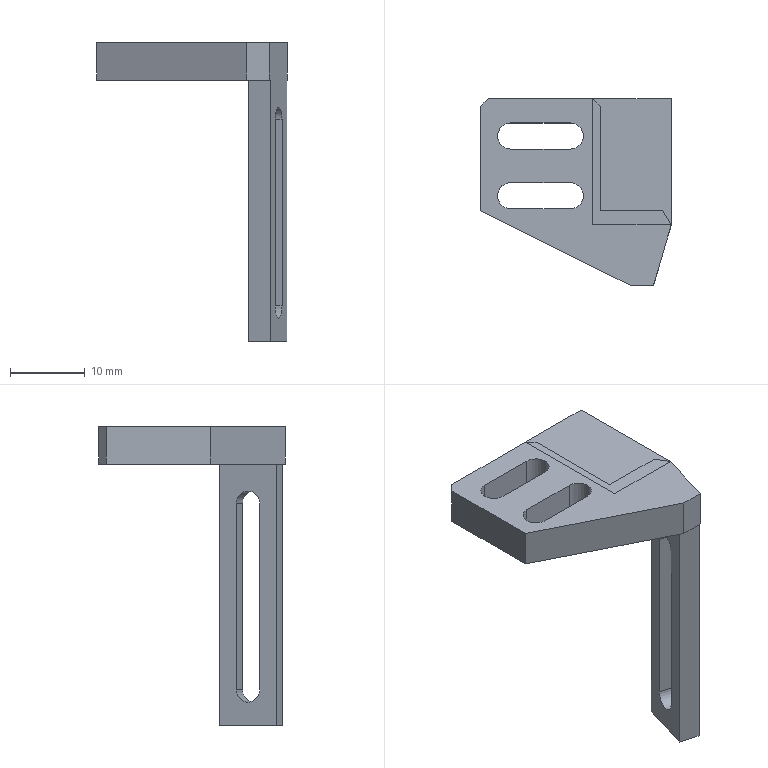Part | NX | 2 solids | 34 faces | box 25.523 x 25 x 40 mm | volume 2991 mm3 | plane 28 | cylinder 6 | commonest cylinder face diameters 3.5 x4 3.3 x2
STEP:
#1=CARTESIAN_POINT('',(12.761,-4.418,0.));
#2=VERTEX_POINT('',#1);
#3=CARTESIAN_POINT('',(2.239,-4.418,0.));
#4=VERTEX_POINT('',#3);
#5=CARTESIAN_POINT('',(7.5,-4.418,0.));
#6=DIRECTION('',(-1.,0.,0.));
#7=VECTOR('',#6,1000.);
#8=LINE('',#5,#7);
#9=EDGE_CURVE('',#2,#4,#8,.T.);
#10=ORIENTED_EDGE('',*,*,#9,.F.);
#11=CARTESIAN_POINT('',(12.761,12.5,0.));
#12=VERTEX_POINT('',#11);
#13=CARTESIAN_POINT('',(12.761,4.041,0.));
#14=DIRECTION('',(0.,-1.,0.));
#15=VECTOR('',#14,1000.);
#16=LINE('',#13,#15);
#17=EDGE_CURVE('',#12,#2,#16,.T.);
#18=ORIENTED_EDGE('',*,*,#17,.F.);
#19=CARTESIAN_POINT('',(2.239,12.5,0.));
#20=VERTEX_POINT('',#19);
#21=CARTESIAN_POINT('',(7.5,12.5,0.));
#22=DIRECTION('',(1.,0.,0.));
#23=VECTOR('',#22,1000.);
#24=LINE('',#21,#23);
#25=EDGE_CURVE('',#20,#12,#24,.T.);
#26=ORIENTED_EDGE('',*,*,#25,.F.);
#27=CARTESIAN_POINT('',(2.239,4.041,0.));
#28=DIRECTION('',(0.,1.,0.));
#29=VECTOR('',#28,1000.);
#30=LINE('',#27,#29);
#31=EDGE_CURVE('',#4,#20,#30,.T.);
#32=ORIENTED_EDGE('',*,*,#31,.F.);
#33=EDGE_LOOP('',(#10,#18,#26,#32));
#34=FACE_BOUND('',#33,.T.);
#35=CARTESIAN_POINT('',(7.5,4.041,0.));
#36=DIRECTION('',(0.,0.,1.));
#37=DIRECTION('',(1.,0.,0.));
#38=AXIS2_PLACEMENT_3D('',#35,#36,#37);
#39=PLANE('',#38);
#40=ADVANCED_FACE('',(#34),#39,.T.);
#41=CARTESIAN_POINT('',(12.761,-4.418,-5.));
#42=VERTEX_POINT('',#41);
#43=CARTESIAN_POINT('',(12.761,-4.418,-5.));
#44=DIRECTION('',(0.,0.,1.));
#45=VECTOR('',#44,1000.);
#46=LINE('',#43,#45);
#47=EDGE_CURVE('',#42,#2,#46,.T.);
#48=ORIENTED_EDGE('',*,*,#47,.T.);
#49=ORIENTED_EDGE('',*,*,#9,.T.);
#50=CARTESIAN_POINT('',(2.239,-4.418,-5.));
#51=VERTEX_POINT('',#50);
#52=CARTESIAN_POINT('',(2.239,-4.418,-5.));
#53=DIRECTION('',(0.,0.,1.));
#54=VECTOR('',#53,1000.);
#55=LINE('',#52,#54);
#56=EDGE_CURVE('',#51,#4,#55,.T.);
#57=ORIENTED_EDGE('',*,*,#56,.F.);
#58=CARTESIAN_POINT('',(7.5,-4.418,-5.));
#59=DIRECTION('',(1.,0.,0.));
#60=VECTOR('',#59,1000.);
#61=LINE('',#58,#60);
#62=EDGE_CURVE('',#51,#42,#61,.T.);
#63=ORIENTED_EDGE('',*,*,#62,.T.);
#64=EDGE_LOOP('',(#48,#49,#57,#63));
#65=FACE_BOUND('',#64,.T.);
#66=CARTESIAN_POINT('',(7.5,-4.418,-5.));
#67=DIRECTION('',(0.,-1.,0.));
#68=DIRECTION('',(0.,0.,-1.));
#69=AXIS2_PLACEMENT_3D('',#66,#67,#68);
#70=PLANE('',#69);
#71=ADVANCED_FACE('',(#65),#70,.T.);
#72=ORIENTED_EDGE('',*,*,#56,.T.);
#73=ORIENTED_EDGE('',*,*,#31,.T.);
#74=CARTESIAN_POINT('',(2.239,12.5,-5.));
#75=VERTEX_POINT('',#74);
#76=CARTESIAN_POINT('',(2.239,12.5,-5.));
#77=DIRECTION('',(0.,0.,1.));
#78=VECTOR('',#77,1000.);
#79=LINE('',#76,#78);
#80=EDGE_CURVE('',#75,#20,#79,.T.);
#81=ORIENTED_EDGE('',*,*,#80,.F.);
#82=CARTESIAN_POINT('',(2.239,4.041,-5.));
#83=DIRECTION('',(0.,-1.,0.));
#84=VECTOR('',#83,1000.);
#85=LINE('',#82,#84);
#86=EDGE_CURVE('',#75,#51,#85,.T.);
#87=ORIENTED_EDGE('',*,*,#86,.T.);
#88=EDGE_LOOP('',(#72,#73,#81,#87));
#89=FACE_BOUND('',#88,.T.);
#90=CARTESIAN_POINT('',(2.239,4.041,-5.));
#91=DIRECTION('',(-1.,0.,0.));
#92=DIRECTION('',(0.,0.,1.));
#93=AXIS2_PLACEMENT_3D('',#90,#91,#92);
#94=PLANE('',#93);
#95=ADVANCED_FACE('',(#89),#94,.T.);
#96=ORIENTED_EDGE('',*,*,#80,.T.);
#97=ORIENTED_EDGE('',*,*,#25,.T.);
#98=CARTESIAN_POINT('',(12.761,12.5,-5.));
#99=VERTEX_POINT('',#98);
#100=CARTESIAN_POINT('',(12.761,12.5,-5.));
#101=DIRECTION('',(0.,0.,1.));
#102=VECTOR('',#101,1000.);
#103=LINE('',#100,#102);
#104=EDGE_CURVE('',#99,#12,#103,.T.);
#105=ORIENTED_EDGE('',*,*,#104,.F.);
#106=CARTESIAN_POINT('',(7.5,12.5,-5.));
#107=DIRECTION('',(-1.,0.,0.));
#108=VECTOR('',#107,1000.);
#109=LINE('',#106,#108);
#110=EDGE_CURVE('',#99,#75,#109,.T.);
#111=ORIENTED_EDGE('',*,*,#110,.T.);
#112=EDGE_LOOP('',(#96,#97,#105,#111));
#113=FACE_BOUND('',#112,.T.);
#114=CARTESIAN_POINT('',(7.5,12.5,-5.));
#115=DIRECTION('',(0.,1.,0.));
#116=DIRECTION('',(0.,0.,1.));
#117=AXIS2_PLACEMENT_3D('',#114,#115,#116);
#118=PLANE('',#117);
#119=ADVANCED_FACE('',(#113),#118,.T.);
#120=CARTESIAN_POINT('',(12.761,4.041,-5.));
#121=DIRECTION('',(0.,1.,0.));
#122=VECTOR('',#121,1000.);
#123=LINE('',#120,#122);
#124=EDGE_CURVE('',#42,#99,#123,.T.);
#125=ORIENTED_EDGE('',*,*,#124,.F.);
#126=ORIENTED_EDGE('',*,*,#62,.F.);
#127=ORIENTED_EDGE('',*,*,#86,.F.);
#128=ORIENTED_EDGE('',*,*,#110,.F.);
#129=EDGE_LOOP('',(#125,#126,#127,#128));
#130=FACE_BOUND('',#129,.T.);
#131=CARTESIAN_POINT('',(7.5,4.041,-5.));
#132=DIRECTION('',(0.,0.,-1.));
#133=DIRECTION('',(-1.,0.,0.));
#134=AXIS2_PLACEMENT_3D('',#131,#132,#133);
#135=PLANE('',#134);
#136=ADVANCED_FACE('',(#130),#135,.T.);
#137=ORIENTED_EDGE('',*,*,#124,.T.);
#138=ORIENTED_EDGE('',*,*,#104,.T.);
#139=ORIENTED_EDGE('',*,*,#17,.T.);
#140=ORIENTED_EDGE('',*,*,#47,.F.);
#141=EDGE_LOOP('',(#137,#138,#139,#140));
#142=FACE_BOUND('',#141,.T.);
#143=CARTESIAN_POINT('',(12.761,4.041,-5.));
#144=DIRECTION('',(1.,0.,0.));
#145=DIRECTION('',(0.,0.,-1.));
#146=AXIS2_PLACEMENT_3D('',#143,#144,#145);
#147=PLANE('',#146);
#148=ADVANCED_FACE('',(#142),#147,.T.);
#149=CLOSED_SHELL('',(#40,#71,#95,#119,#136,#148));
#150=MANIFOLD_SOLID_BREP('',#149);
#151=CARTESIAN_POINT('',(10.367,-12.5,0.));
#152=VERTEX_POINT('',#151);
#153=CARTESIAN_POINT('',(7.239,-12.5,0.));
#154=VERTEX_POINT('',#153);
#155=CARTESIAN_POINT('',(-12.761,-12.5,0.));
#156=DIRECTION('',(-1.,0.,0.));
#157=VECTOR('',#156,1000.);
#158=LINE('',#155,#157);
#159=EDGE_CURVE('',#152,#154,#158,.T.);
#160=ORIENTED_EDGE('',*,*,#159,.T.);
#161=CARTESIAN_POINT('',(7.239,-12.5,-5.));
#162=VERTEX_POINT('',#161);
#163=CARTESIAN_POINT('',(7.239,-12.5,-5.));
#164=DIRECTION('',(0.,0.,-1.));
#165=VECTOR('',#164,1000.);
#166=LINE('',#163,#165);
#167=EDGE_CURVE('',#154,#162,#166,.T.);
#168=ORIENTED_EDGE('',*,*,#167,.T.);
#169=CARTESIAN_POINT('',(10.367,-12.5,-5.));
#170=VERTEX_POINT('',#169);
#171=CARTESIAN_POINT('',(-12.761,-12.5,-5.));
#172=DIRECTION('',(-1.,0.,0.));
#173=VECTOR('',#172,1000.);
#174=LINE('',#171,#173);
#175=EDGE_CURVE('',#170,#162,#174,.T.);
#176=ORIENTED_EDGE('',*,*,#175,.F.);
#177=CARTESIAN_POINT('',(10.367,-12.5,0.));
#178=DIRECTION('',(0.,0.,-1.));
#179=VECTOR('',#178,1000.);
#180=LINE('',#177,#179);
#181=EDGE_CURVE('',#152,#170,#180,.T.);
#182=ORIENTED_EDGE('',*,*,#181,.F.);
#183=EDGE_LOOP('',(#160,#168,#176,#182));
#184=FACE_BOUND('',#183,.T.);
#185=CARTESIAN_POINT('',(-12.761,-12.5,-5.));
#186=DIRECTION('',(0.,1.,0.));
#187=DIRECTION('',(-1.,0.,0.));
#188=AXIS2_PLACEMENT_3D('',#185,#186,#187);
#189=PLANE('',#188);
#190=ADVANCED_FACE('',(#184),#189,.F.);
#191=CARTESIAN_POINT('',(8.251,-9.082,-10.25));
#192=VERTEX_POINT('',#191);
#193=CARTESIAN_POINT('',(8.251,-9.082,-35.25));
#194=VERTEX_POINT('',#193);
#195=CARTESIAN_POINT('',(8.251,-9.082,-35.));
#196=DIRECTION('',(0.,0.,-1.));
#197=VECTOR('',#196,1000.);
#198=LINE('',#195,#197);
#199=EDGE_CURVE('',#192,#194,#198,.T.);
#200=ORIENTED_EDGE('',*,*,#199,.T.);
#201=CARTESIAN_POINT('',(9.188,-5.918,-35.25));
#202=VERTEX_POINT('',#201);
#203=CARTESIAN_POINT('',(8.72,-7.5,-35.25));
#204=DIRECTION('',(0.9588,-0.284,0.));
#205=DIRECTION('',(-0.284,-0.9588,0.));
#206=AXIS2_PLACEMENT_3D('',#203,#204,#205);
#207=CIRCLE('',#206,1.65);
#208=EDGE_CURVE('',#194,#202,#207,.T.);
#209=ORIENTED_EDGE('',*,*,#208,.T.);
#210=CARTESIAN_POINT('',(9.188,-5.918,-10.25));
#211=VERTEX_POINT('',#210);
#212=CARTESIAN_POINT('',(9.188,-5.918,-35.));
#213=DIRECTION('',(0.,0.,1.));
#214=VECTOR('',#213,1000.);
#215=LINE('',#212,#214);
#216=EDGE_CURVE('',#202,#211,#215,.T.);
#217=ORIENTED_EDGE('',*,*,#216,.T.);
#218=CARTESIAN_POINT('',(8.72,-7.5,-10.25));
#219=DIRECTION('',(0.9588,-0.284,0.));
#220=DIRECTION('',(-0.284,-0.9588,0.));
#221=AXIS2_PLACEMENT_3D('',#218,#219,#220);
#222=CIRCLE('',#221,1.65);
#223=EDGE_CURVE('',#211,#192,#222,.T.);
#224=ORIENTED_EDGE('',*,*,#223,.T.);
#225=EDGE_LOOP('',(#200,#209,#217,#224));
#226=FACE_BOUND('',#225,.T.);
#227=CARTESIAN_POINT('',(7.593,-11.302,-5.));
#228=VERTEX_POINT('',#227);
#229=CARTESIAN_POINT('',(9.846,-3.698,-5.));
#230=VERTEX_POINT('',#229);
#231=CARTESIAN_POINT('',(13.163,7.5,-5.));
#232=DIRECTION('',(0.284,0.9588,0.));
#233=VECTOR('',#232,1000.);
#234=LINE('',#231,#233);
#235=EDGE_CURVE('',#228,#230,#234,.T.);
#236=ORIENTED_EDGE('',*,*,#235,.T.);
#237=CARTESIAN_POINT('',(9.846,-3.698,-40.));
#238=VERTEX_POINT('',#237);
#239=CARTESIAN_POINT('',(9.846,-3.698,0.));
#240=DIRECTION('',(0.,0.,1.));
#241=VECTOR('',#240,1000.);
#242=LINE('',#239,#241);
#243=EDGE_CURVE('',#238,#230,#242,.T.);
#244=ORIENTED_EDGE('',*,*,#243,.F.);
#245=CARTESIAN_POINT('',(7.593,-11.302,-40.));
#246=VERTEX_POINT('',#245);
#247=CARTESIAN_POINT('',(9.856,-3.665,-40.));
#248=DIRECTION('',(-0.284,-0.9588,0.));
#249=VECTOR('',#248,1000.);
#250=LINE('',#247,#249);
#251=EDGE_CURVE('',#238,#246,#250,.T.);
#252=ORIENTED_EDGE('',*,*,#251,.T.);
#253=CARTESIAN_POINT('',(7.593,-11.302,0.));
#254=DIRECTION('',(0.,0.,1.));
#255=VECTOR('',#254,1000.);
#256=LINE('',#253,#255);
#257=EDGE_CURVE('',#246,#228,#256,.T.);
#258=ORIENTED_EDGE('',*,*,#257,.T.);
#259=EDGE_LOOP('',(#236,#244,#252,#258));
#260=FACE_BOUND('',#259,.T.);
#261=CARTESIAN_POINT('',(13.163,7.5,-35.));
#262=DIRECTION('',(0.9588,-0.284,0.));
#263=DIRECTION('',(0.284,0.9588,0.));
#264=AXIS2_PLACEMENT_3D('',#261,#262,#263);
#265=PLANE('',#264);
#266=ADVANCED_FACE('',(#226,#260),#265,.F.);
#267=CARTESIAN_POINT('',(12.065,-6.77,-35.25));
#268=VERTEX_POINT('',#267);
#269=CARTESIAN_POINT('',(12.065,-6.77,-10.25));
#270=VERTEX_POINT('',#269);
#271=CARTESIAN_POINT('',(12.065,-6.77,-35.25));
#272=DIRECTION('',(0.,0.,1.));
#273=VECTOR('',#272,1000.);
#274=LINE('',#271,#273);
#275=EDGE_CURVE('',#268,#270,#274,.T.);
#276=ORIENTED_EDGE('',*,*,#275,.F.);
#277=CARTESIAN_POINT('',(11.127,-9.934,-35.25));
#278=VERTEX_POINT('',#277);
#279=CARTESIAN_POINT('',(11.596,-8.352,-35.25));
#280=DIRECTION('',(0.9588,-0.284,0.));
#281=DIRECTION('',(-0.284,-0.9588,0.));
#282=AXIS2_PLACEMENT_3D('',#279,#280,#281);
#283=CIRCLE('',#282,1.65);
#284=EDGE_CURVE('',#278,#268,#283,.T.);
#285=ORIENTED_EDGE('',*,*,#284,.F.);
#286=CARTESIAN_POINT('',(11.127,-9.934,-10.25));
#287=VERTEX_POINT('',#286);
#288=CARTESIAN_POINT('',(11.127,-9.934,-35.25));
#289=DIRECTION('',(0.,0.,-1.));
#290=VECTOR('',#289,1000.);
#291=LINE('',#288,#290);
#292=EDGE_CURVE('',#287,#278,#291,.T.);
#293=ORIENTED_EDGE('',*,*,#292,.F.);
#294=CARTESIAN_POINT('',(11.596,-8.352,-10.25));
#295=DIRECTION('',(0.9588,-0.284,0.));
#296=DIRECTION('',(-0.284,-0.9588,0.));
#297=AXIS2_PLACEMENT_3D('',#294,#295,#296);
#298=CIRCLE('',#297,1.65);
#299=EDGE_CURVE('',#270,#287,#298,.T.);
#300=ORIENTED_EDGE('',*,*,#299,.F.);
#301=EDGE_LOOP('',(#276,#285,#293,#300));
#302=FACE_BOUND('',#301,.T.);
#303=CARTESIAN_POINT('',(12.761,-4.418,-5.));
#304=VERTEX_POINT('',#303);
#305=CARTESIAN_POINT('',(12.722,-4.55,-5.));
#306=VERTEX_POINT('',#305);
#307=CARTESIAN_POINT('',(13.33,-2.5,-5.));
#308=DIRECTION('',(0.284,0.9588,0.));
#309=VECTOR('',#308,1000.);
#310=LINE('',#307,#309);
#311=EDGE_CURVE('',#304,#306,#310,.F.);
#312=ORIENTED_EDGE('',*,*,#311,.F.);
#313=CARTESIAN_POINT('',(12.761,-4.418,0.));
#314=VERTEX_POINT('',#313);
#315=CARTESIAN_POINT('',(12.761,-4.418,0.));
#316=DIRECTION('',(0.,0.,1.));
#317=VECTOR('',#316,1000.);
#318=LINE('',#315,#317);
#319=EDGE_CURVE('',#304,#314,#318,.T.);
#320=ORIENTED_EDGE('',*,*,#319,.T.);
#321=CARTESIAN_POINT('',(13.33,-2.5,0.));
#322=DIRECTION('',(0.284,0.9588,0.));
#323=VECTOR('',#322,1000.);
#324=LINE('',#321,#323);
#325=EDGE_CURVE('',#152,#314,#324,.T.);
#326=ORIENTED_EDGE('',*,*,#325,.F.);
#327=ORIENTED_EDGE('',*,*,#181,.T.);
#328=CARTESIAN_POINT('',(10.47,-12.154,-5.));
#329=VERTEX_POINT('',#328);
#330=CARTESIAN_POINT('',(13.33,-2.5,-5.));
#331=DIRECTION('',(-0.284,-0.9588,0.));
#332=VECTOR('',#331,1000.);
#333=LINE('',#330,#332);
#334=EDGE_CURVE('',#170,#329,#333,.F.);
#335=ORIENTED_EDGE('',*,*,#334,.T.);
#336=CARTESIAN_POINT('',(10.47,-12.154,-40.));
#337=VERTEX_POINT('',#336);
#338=CARTESIAN_POINT('',(10.47,-12.154,0.));
#339=DIRECTION('',(0.,0.,1.));
#340=VECTOR('',#339,1000.);
#341=LINE('',#338,#340);
#342=EDGE_CURVE('',#337,#329,#341,.T.);
#343=ORIENTED_EDGE('',*,*,#342,.F.);
#344=CARTESIAN_POINT('',(12.722,-4.55,-40.));
#345=VERTEX_POINT('',#344);
#346=CARTESIAN_POINT('',(12.732,-4.517,-40.));
#347=DIRECTION('',(0.284,0.9588,0.));
#348=VECTOR('',#347,1000.);
#349=LINE('',#346,#348);
#350=EDGE_CURVE('',#337,#345,#349,.T.);
#351=ORIENTED_EDGE('',*,*,#350,.T.);
#352=CARTESIAN_POINT('',(12.722,-4.55,0.));
#353=DIRECTION('',(0.,0.,1.));
#354=VECTOR('',#353,1000.);
#355=LINE('',#352,#354);
#356=EDGE_CURVE('',#345,#306,#355,.T.);
#357=ORIENTED_EDGE('',*,*,#356,.T.);
#358=EDGE_LOOP('',(#312,#320,#326,#327,#335,#343,#351,#357));
#359=FACE_BOUND('',#358,.T.);
#360=CARTESIAN_POINT('',(13.33,-2.5,0.));
#361=DIRECTION('',(-0.9588,0.284,0.));
#362=DIRECTION('',(-0.284,-0.9588,0.));
#363=AXIS2_PLACEMENT_3D('',#360,#361,#362);
#364=PLANE('',#363);
#365=ADVANCED_FACE('',(#302,#359),#364,.F.);
#366=CARTESIAN_POINT('',(-0.7615,-2.25,-5.));
#367=VERTEX_POINT('',#366);
#368=CARTESIAN_POINT('',(-8.761,-2.25,-5.));
#369=VERTEX_POINT('',#368);
#370=CARTESIAN_POINT('',(-0.7615,-2.25,-5.));
#371=DIRECTION('',(-1.,0.,0.));
#372=VECTOR('',#371,1000.);
#373=LINE('',#370,#372);
#374=EDGE_CURVE('',#367,#369,#373,.T.);
#375=ORIENTED_EDGE('',*,*,#374,.F.);
#376=CARTESIAN_POINT('',(-0.7615,1.25,-5.));
#377=VERTEX_POINT('',#376);
#378=CARTESIAN_POINT('',(-0.7615,-0.5,-5.));
#379=DIRECTION('',(0.,0.,-1.));
#380=DIRECTION('',(0.,-1.,0.));
#381=AXIS2_PLACEMENT_3D('',#378,#379,#380);
#382=CIRCLE('',#381,1.75);
#383=EDGE_CURVE('',#377,#367,#382,.T.);
#384=ORIENTED_EDGE('',*,*,#383,.F.);
#385=CARTESIAN_POINT('',(-8.761,1.25,-5.));
#386=VERTEX_POINT('',#385);
#387=CARTESIAN_POINT('',(-0.7615,1.25,-5.));
#388=DIRECTION('',(1.,0.,0.));
#389=VECTOR('',#388,1000.);
#390=LINE('',#387,#389);
#391=EDGE_CURVE('',#386,#377,#390,.T.);
#392=ORIENTED_EDGE('',*,*,#391,.F.);
#393=CARTESIAN_POINT('',(-8.761,-0.5,-5.));
#394=DIRECTION('',(0.,0.,-1.));
#395=DIRECTION('',(0.,-1.,0.));
#396=AXIS2_PLACEMENT_3D('',#393,#394,#395);
#397=CIRCLE('',#396,1.75);
#398=EDGE_CURVE('',#369,#386,#397,.T.);
#399=ORIENTED_EDGE('',*,*,#398,.F.);
#400=EDGE_LOOP('',(#375,#384,#392,#399));
#401=FACE_BOUND('',#400,.T.);
#402=CARTESIAN_POINT('',(-0.7615,5.75,-5.));
#403=VERTEX_POINT('',#402);
#404=CARTESIAN_POINT('',(-8.761,5.75,-5.));
#405=VERTEX_POINT('',#404);
#406=CARTESIAN_POINT('',(-0.7615,5.75,-5.));
#407=DIRECTION('',(-1.,0.,0.));
#408=VECTOR('',#407,1000.);
#409=LINE('',#406,#408);
#410=EDGE_CURVE('',#403,#405,#409,.T.);
#411=ORIENTED_EDGE('',*,*,#410,.F.);
#412=CARTESIAN_POINT('',(-0.7615,9.25,-5.));
#413=VERTEX_POINT('',#412);
#414=CARTESIAN_POINT('',(-0.7615,7.5,-5.));
#415=DIRECTION('',(0.,0.,-1.));
#416=DIRECTION('',(0.,-1.,0.));
#417=AXIS2_PLACEMENT_3D('',#414,#415,#416);
#418=CIRCLE('',#417,1.75);
#419=EDGE_CURVE('',#413,#403,#418,.T.);
#420=ORIENTED_EDGE('',*,*,#419,.F.);
#421=CARTESIAN_POINT('',(-8.761,9.25,-5.));
#422=VERTEX_POINT('',#421);
#423=CARTESIAN_POINT('',(-0.7615,9.25,-5.));
#424=DIRECTION('',(1.,0.,0.));
#425=VECTOR('',#424,1000.);
#426=LINE('',#423,#425);
#427=EDGE_CURVE('',#422,#413,#426,.T.);
#428=ORIENTED_EDGE('',*,*,#427,.F.);
#429=CARTESIAN_POINT('',(-8.761,7.5,-5.));
#430=DIRECTION('',(0.,0.,-1.));
#431=DIRECTION('',(0.,-1.,0.));
#432=AXIS2_PLACEMENT_3D('',#429,#430,#431);
#433=CIRCLE('',#432,1.75);
#434=EDGE_CURVE('',#405,#422,#433,.T.);
#435=ORIENTED_EDGE('',*,*,#434,.F.);
#436=EDGE_LOOP('',(#411,#420,#428,#435));
#437=FACE_BOUND('',#436,.T.);
#438=ORIENTED_EDGE('',*,*,#175,.T.);
#439=CARTESIAN_POINT('',(-12.761,-2.5,-5.));
#440=VERTEX_POINT('',#439);
#441=CARTESIAN_POINT('',(-12.761,-2.5,-5.));
#442=DIRECTION('',(-0.8944,0.4472,0.));
#443=VECTOR('',#442,1000.);
#444=LINE('',#441,#443);
#445=EDGE_CURVE('',#162,#440,#444,.T.);
#446=ORIENTED_EDGE('',*,*,#445,.T.);
#447=CARTESIAN_POINT('',(-12.761,11.5,-5.));
#448=VERTEX_POINT('',#447);
#449=CARTESIAN_POINT('',(-12.761,12.5,-5.));
#450=DIRECTION('',(0.,1.,0.));
#451=VECTOR('',#450,1000.);
#452=LINE('',#449,#451);
#453=EDGE_CURVE('',#440,#448,#452,.T.);
#454=ORIENTED_EDGE('',*,*,#453,.T.);
#455=CARTESIAN_POINT('',(-11.761,12.5,-5.));
#456=VERTEX_POINT('',#455);
#457=CARTESIAN_POINT('',(-11.761,12.5,-5.));
#458=DIRECTION('',(0.7071,0.7071,0.));
#459=VECTOR('',#458,1000.);
#460=LINE('',#457,#459);
#461=EDGE_CURVE('',#448,#456,#460,.T.);
#462=ORIENTED_EDGE('',*,*,#461,.T.);
#463=CARTESIAN_POINT('',(2.239,12.5,-5.));
#464=VERTEX_POINT('',#463);
#465=CARTESIAN_POINT('',(17.239,12.5,-5.));
#466=DIRECTION('',(1.,0.,0.));
#467=VECTOR('',#466,1000.);
#468=LINE('',#465,#467);
#469=EDGE_CURVE('',#456,#464,#468,.T.);
#470=ORIENTED_EDGE('',*,*,#469,.T.);
#471=CARTESIAN_POINT('',(3.239,11.5,-5.));
#472=VERTEX_POINT('',#471);
#473=CARTESIAN_POINT('',(2.239,12.5,-5.));
#474=DIRECTION('',(0.7071,-0.7071,0.));
#475=VECTOR('',#474,1000.);
#476=LINE('',#473,#475);
#477=EDGE_CURVE('',#464,#472,#476,.T.);
#478=ORIENTED_EDGE('',*,*,#477,.T.);
#479=CARTESIAN_POINT('',(3.239,-2.5,-5.));
#480=VERTEX_POINT('',#479);
#481=CARTESIAN_POINT('',(3.239,-12.5,-5.));
#482=DIRECTION('',(0.,-1.,0.));
#483=VECTOR('',#482,1000.);
#484=LINE('',#481,#483);
#485=EDGE_CURVE('',#472,#480,#484,.T.);
#486=ORIENTED_EDGE('',*,*,#485,.T.);
#487=CARTESIAN_POINT('',(11.586,-2.5,-5.));
#488=VERTEX_POINT('',#487);
#489=CARTESIAN_POINT('',(-12.761,-2.5,-5.));
#490=DIRECTION('',(1.,0.,0.));
#491=VECTOR('',#490,1000.);
#492=LINE('',#489,#491);
#493=EDGE_CURVE('',#480,#488,#492,.T.);
#494=ORIENTED_EDGE('',*,*,#493,.T.);
#495=CARTESIAN_POINT('',(11.586,-2.5,-5.));
#496=DIRECTION('',(0.5225,-0.8526,0.));
#497=VECTOR('',#496,1000.);
#498=LINE('',#495,#497);
#499=EDGE_CURVE('',#488,#304,#498,.T.);
#500=ORIENTED_EDGE('',*,*,#499,.T.);
#501=ORIENTED_EDGE('',*,*,#311,.T.);
#502=CARTESIAN_POINT('',(17.516,-5.97,-5.));
#503=DIRECTION('',(-0.9588,0.284,0.));
#504=VECTOR('',#503,1000.);
#505=LINE('',#502,#504);
#506=EDGE_CURVE('',#306,#230,#505,.T.);
#507=ORIENTED_EDGE('',*,*,#506,.T.);
#508=ORIENTED_EDGE('',*,*,#235,.F.);
#509=CARTESIAN_POINT('',(15.264,-13.574,-5.));
#510=DIRECTION('',(-0.9588,0.284,0.));
#511=VECTOR('',#510,1000.);
#512=LINE('',#509,#511);
#513=EDGE_CURVE('',#329,#228,#512,.T.);
#514=ORIENTED_EDGE('',*,*,#513,.F.);
#515=ORIENTED_EDGE('',*,*,#334,.F.);
#516=EDGE_LOOP('',(#438,#446,#454,#462,#470,#478,#486,#494,#500,#501,#507,#508,#514,#515));
#517=FACE_BOUND('',#516,.T.);
#518=CARTESIAN_POINT('',(-12.761,-12.5,-5.));
#519=DIRECTION('',(0.,0.,1.));
#520=DIRECTION('',(0.,-1.,0.));
#521=AXIS2_PLACEMENT_3D('',#518,#519,#520);
#522=PLANE('',#521);
#523=ADVANCED_FACE('',(#401,#437,#517),#522,.F.);
#524=ORIENTED_EDGE('',*,*,#453,.F.);
#525=CARTESIAN_POINT('',(-12.761,-2.5,0.));
#526=VERTEX_POINT('',#525);
#527=CARTESIAN_POINT('',(-12.761,-2.5,-5.));
#528=DIRECTION('',(0.,0.,1.));
#529=VECTOR('',#528,1000.);
#530=LINE('',#527,#529);
#531=EDGE_CURVE('',#440,#526,#530,.T.);
#532=ORIENTED_EDGE('',*,*,#531,.T.);
#533=CARTESIAN_POINT('',(-12.761,11.5,0.));
#534=VERTEX_POINT('',#533);
#535=CARTESIAN_POINT('',(-12.761,12.5,0.));
#536=DIRECTION('',(0.,1.,0.));
#537=VECTOR('',#536,1000.);
#538=LINE('',#535,#537);
#539=EDGE_CURVE('',#526,#534,#538,.T.);
#540=ORIENTED_EDGE('',*,*,#539,.T.);
#541=CARTESIAN_POINT('',(-12.761,11.5,-5.));
#542=DIRECTION('',(0.,0.,-1.));
#543=VECTOR('',#542,1000.);
#544=LINE('',#541,#543);
#545=EDGE_CURVE('',#534,#448,#544,.T.);
#546=ORIENTED_EDGE('',*,*,#545,.T.);
#547=EDGE_LOOP('',(#524,#532,#540,#546));
#548=FACE_BOUND('',#547,.T.);
#549=CARTESIAN_POINT('',(-12.761,12.5,-5.));
#550=DIRECTION('',(1.,0.,0.));
#551=DIRECTION('',(0.,1.,0.));
#552=AXIS2_PLACEMENT_3D('',#549,#550,#551);
#553=PLANE('',#552);
#554=ADVANCED_FACE('',(#548),#553,.F.);
#555=ORIENTED_EDGE('',*,*,#469,.F.);
#556=CARTESIAN_POINT('',(-11.761,12.5,0.));
#557=VERTEX_POINT('',#556);
#558=CARTESIAN_POINT('',(-11.761,12.5,-5.));
#559=DIRECTION('',(0.,0.,1.));
#560=VECTOR('',#559,1000.);
#561=LINE('',#558,#560);
#562=EDGE_CURVE('',#456,#557,#561,.T.);
#563=ORIENTED_EDGE('',*,*,#562,.T.);
#564=CARTESIAN_POINT('',(2.239,12.5,0.));
#565=VERTEX_POINT('',#564);
#566=CARTESIAN_POINT('',(17.239,12.5,0.));
#567=DIRECTION('',(1.,0.,0.));
#568=VECTOR('',#567,1000.);
#569=LINE('',#566,#568);
#570=EDGE_CURVE('',#557,#565,#569,.T.);
#571=ORIENTED_EDGE('',*,*,#570,.T.);
#572=CARTESIAN_POINT('',(2.239,12.5,-5.));
#573=DIRECTION('',(0.,0.,-1.));
#574=VECTOR('',#573,1000.);
#575=LINE('',#572,#574);
#576=EDGE_CURVE('',#565,#464,#575,.T.);
#577=ORIENTED_EDGE('',*,*,#576,.T.);
#578=EDGE_LOOP('',(#555,#563,#571,#577));
#579=FACE_BOUND('',#578,.T.);
#580=CARTESIAN_POINT('',(17.239,12.5,-5.));
#581=DIRECTION('',(0.,-1.,0.));
#582=DIRECTION('',(1.,0.,0.));
#583=AXIS2_PLACEMENT_3D('',#580,#581,#582);
#584=PLANE('',#583);
#585=ADVANCED_FACE('',(#579),#584,.F.);
#586=ORIENTED_EDGE('',*,*,#539,.F.);
#587=CARTESIAN_POINT('',(-8.761,-4.5,0.));
#588=DIRECTION('',(0.8944,-0.4472,0.));
#589=VECTOR('',#588,1000.);
#590=LINE('',#587,#589);
#591=EDGE_CURVE('',#526,#154,#590,.T.);
#592=ORIENTED_EDGE('',*,*,#591,.T.);
#593=ORIENTED_EDGE('',*,*,#159,.F.);
#594=ORIENTED_EDGE('',*,*,#325,.T.);
#595=CARTESIAN_POINT('',(11.586,-2.5,0.));
#596=VERTEX_POINT('',#595);
#597=CARTESIAN_POINT('',(9.394,1.077,0.));
#598=DIRECTION('',(-0.5225,0.8526,0.));
#599=VECTOR('',#598,1000.);
#600=LINE('',#597,#599);
#601=EDGE_CURVE('',#314,#596,#600,.T.);
#602=ORIENTED_EDGE('',*,*,#601,.T.);
#603=CARTESIAN_POINT('',(3.239,-2.5,0.));
#604=VERTEX_POINT('',#603);
#605=CARTESIAN_POINT('',(17.239,-2.5,0.));
#606=DIRECTION('',(-1.,0.,0.));
#607=VECTOR('',#606,1000.);
#608=LINE('',#605,#607);
#609=EDGE_CURVE('',#596,#604,#608,.T.);
#610=ORIENTED_EDGE('',*,*,#609,.T.);
#611=CARTESIAN_POINT('',(3.239,11.5,0.));
#612=VERTEX_POINT('',#611);
#613=CARTESIAN_POINT('',(3.239,12.5,0.));
#614=DIRECTION('',(0.,1.,0.));
#615=VECTOR('',#614,1000.);
#616=LINE('',#613,#615);
#617=EDGE_CURVE('',#604,#612,#616,.T.);
#618=ORIENTED_EDGE('',*,*,#617,.T.);
#619=CARTESIAN_POINT('',(7.239,7.5,0.));
#620=DIRECTION('',(-0.7071,0.7071,0.));
#621=VECTOR('',#620,1000.);
#622=LINE('',#619,#621);
#623=EDGE_CURVE('',#612,#565,#622,.T.);
#624=ORIENTED_EDGE('',*,*,#623,.T.);
#625=ORIENTED_EDGE('',*,*,#570,.F.);
#626=CARTESIAN_POINT('',(-24.761,-0.5,0.));
#627=DIRECTION('',(-0.7071,-0.7071,0.));
#628=VECTOR('',#627,1000.);
#629=LINE('',#626,#628);
#630=EDGE_CURVE('',#557,#534,#629,.T.);
#631=ORIENTED_EDGE('',*,*,#630,.T.);
#632=EDGE_LOOP('',(#586,#592,#593,#594,#602,#610,#618,#624,#625,#631));
#633=FACE_BOUND('',#632,.T.);
#634=CARTESIAN_POINT('',(-0.7615,1.25,0.));
#635=VERTEX_POINT('',#634);
#636=CARTESIAN_POINT('',(-0.7615,-2.25,0.));
#637=VERTEX_POINT('',#636);
#638=CARTESIAN_POINT('',(-0.7615,-0.5,0.));
#639=DIRECTION('',(0.,0.,-1.));
#640=DIRECTION('',(0.,-1.,0.));
#641=AXIS2_PLACEMENT_3D('',#638,#639,#640);
#642=CIRCLE('',#641,1.75);
#643=EDGE_CURVE('',#635,#637,#642,.T.);
#644=ORIENTED_EDGE('',*,*,#643,.T.);
#645=CARTESIAN_POINT('',(-8.761,-2.25,0.));
#646=VERTEX_POINT('',#645);
#647=CARTESIAN_POINT('',(-0.7615,-2.25,0.));
#648=DIRECTION('',(-1.,0.,0.));
#649=VECTOR('',#648,1000.);
#650=LINE('',#647,#649);
#651=EDGE_CURVE('',#637,#646,#650,.T.);
#652=ORIENTED_EDGE('',*,*,#651,.T.);
#653=CARTESIAN_POINT('',(-8.761,1.25,0.));
#654=VERTEX_POINT('',#653);
#655=CARTESIAN_POINT('',(-8.761,-0.5,0.));
#656=DIRECTION('',(0.,0.,-1.));
#657=DIRECTION('',(0.,-1.,0.));
#658=AXIS2_PLACEMENT_3D('',#655,#656,#657);
#659=CIRCLE('',#658,1.75);
#660=EDGE_CURVE('',#646,#654,#659,.T.);
#661=ORIENTED_EDGE('',*,*,#660,.T.);
#662=CARTESIAN_POINT('',(-0.7615,1.25,0.));
#663=DIRECTION('',(1.,0.,0.));
#664=VECTOR('',#663,1000.);
#665=LINE('',#662,#664);
#666=EDGE_CURVE('',#654,#635,#665,.T.);
#667=ORIENTED_EDGE('',*,*,#666,.T.);
#668=EDGE_LOOP('',(#644,#652,#661,#667));
#669=FACE_BOUND('',#668,.T.);
#670=CARTESIAN_POINT('',(-0.7615,9.25,0.));
#671=VERTEX_POINT('',#670);
#672=CARTESIAN_POINT('',(-0.7615,5.75,0.));
#673=VERTEX_POINT('',#672);
#674=CARTESIAN_POINT('',(-0.7615,7.5,0.));
#675=DIRECTION('',(0.,0.,-1.));
#676=DIRECTION('',(0.,-1.,0.));
#677=AXIS2_PLACEMENT_3D('',#674,#675,#676);
#678=CIRCLE('',#677,1.75);
#679=EDGE_CURVE('',#671,#673,#678,.T.);
#680=ORIENTED_EDGE('',*,*,#679,.T.);
#681=CARTESIAN_POINT('',(-8.761,5.75,0.));
#682=VERTEX_POINT('',#681);
#683=CARTESIAN_POINT('',(-0.7615,5.75,0.));
#684=DIRECTION('',(-1.,0.,0.));
#685=VECTOR('',#684,1000.);
#686=LINE('',#683,#685);
#687=EDGE_CURVE('',#673,#682,#686,.T.);
#688=ORIENTED_EDGE('',*,*,#687,.T.);
#689=CARTESIAN_POINT('',(-8.761,9.25,0.));
#690=VERTEX_POINT('',#689);
#691=CARTESIAN_POINT('',(-8.761,7.5,0.));
#692=DIRECTION('',(0.,0.,-1.));
#693=DIRECTION('',(0.,-1.,0.));
#694=AXIS2_PLACEMENT_3D('',#691,#692,#693);
#695=CIRCLE('',#694,1.75);
#696=EDGE_CURVE('',#682,#690,#695,.T.);
#697=ORIENTED_EDGE('',*,*,#696,.T.);
#698=CARTESIAN_POINT('',(-0.7615,9.25,0.));
#699=DIRECTION('',(1.,0.,0.));
#700=VECTOR('',#699,1000.);
#701=LINE('',#698,#700);
#702=EDGE_CURVE('',#690,#671,#701,.T.);
#703=ORIENTED_EDGE('',*,*,#702,.T.);
#704=EDGE_LOOP('',(#680,#688,#697,#703));
#705=FACE_BOUND('',#704,.T.);
#706=CARTESIAN_POINT('',(-12.761,-12.5,0.));
#707=DIRECTION('',(0.,0.,1.));
#708=DIRECTION('',(0.,-1.,0.));
#709=AXIS2_PLACEMENT_3D('',#706,#707,#708);
#710=PLANE('',#709);
#711=ADVANCED_FACE('',(#633,#669,#705),#710,.T.);
#712=ORIENTED_EDGE('',*,*,#485,.F.);
#713=CARTESIAN_POINT('',(3.239,11.5,0.));
#714=DIRECTION('',(0.,0.,1.));
#715=VECTOR('',#714,1000.);
#716=LINE('',#713,#715);
#717=EDGE_CURVE('',#472,#612,#716,.T.);
#718=ORIENTED_EDGE('',*,*,#717,.T.);
#719=ORIENTED_EDGE('',*,*,#617,.F.);
#720=CARTESIAN_POINT('',(3.239,-2.5,0.));
#721=DIRECTION('',(0.,0.,-1.));
#722=VECTOR('',#721,1000.);
#723=LINE('',#720,#722);
#724=EDGE_CURVE('',#604,#480,#723,.T.);
#725=ORIENTED_EDGE('',*,*,#724,.T.);
#726=EDGE_LOOP('',(#712,#718,#719,#725));
#727=FACE_BOUND('',#726,.T.);
#728=CARTESIAN_POINT('',(3.239,12.5,0.));
#729=DIRECTION('',(-1.,0.,0.));
#730=DIRECTION('',(0.,-1.,0.));
#731=AXIS2_PLACEMENT_3D('',#728,#729,#730);
#732=PLANE('',#731);
#733=ADVANCED_FACE('',(#727),#732,.F.);
#734=ORIENTED_EDGE('',*,*,#609,.F.);
#735=CARTESIAN_POINT('',(11.586,-2.5,0.));
#736=DIRECTION('',(0.,0.,-1.));
#737=VECTOR('',#736,1000.);
#738=LINE('',#735,#737);
#739=EDGE_CURVE('',#596,#488,#738,.T.);
#740=ORIENTED_EDGE('',*,*,#739,.T.);
#741=ORIENTED_EDGE('',*,*,#493,.F.);
#742=ORIENTED_EDGE('',*,*,#724,.F.);
#743=EDGE_LOOP('',(#734,#740,#741,#742));
#744=FACE_BOUND('',#743,.T.);
#745=CARTESIAN_POINT('',(17.239,-2.5,0.));
#746=DIRECTION('',(0.,-1.,0.));
#747=DIRECTION('',(1.,0.,0.));
#748=AXIS2_PLACEMENT_3D('',#745,#746,#747);
#749=PLANE('',#748);
#750=ADVANCED_FACE('',(#744),#749,.F.);
#751=ORIENTED_EDGE('',*,*,#419,.T.);
#752=CARTESIAN_POINT('',(-0.7615,5.75,0.));
#753=DIRECTION('',(0.,0.,-1.));
#754=VECTOR('',#753,1000.);
#755=LINE('',#752,#754);
#756=EDGE_CURVE('',#673,#403,#755,.T.);
#757=ORIENTED_EDGE('',*,*,#756,.F.);
#758=ORIENTED_EDGE('',*,*,#679,.F.);
#759=CARTESIAN_POINT('',(-0.7615,9.25,0.));
#760=DIRECTION('',(0.,0.,-1.));
#761=VECTOR('',#760,1000.);
#762=LINE('',#759,#761);
#763=EDGE_CURVE('',#671,#413,#762,.T.);
#764=ORIENTED_EDGE('',*,*,#763,.T.);
#765=EDGE_LOOP('',(#751,#757,#758,#764));
#766=FACE_BOUND('',#765,.T.);
#767=CARTESIAN_POINT('',(-0.7615,7.5,0.));
#768=DIRECTION('',(0.,0.,-1.));
#769=DIRECTION('',(0.,1.,0.));
#770=AXIS2_PLACEMENT_3D('',#767,#768,#769);
#771=CYLINDRICAL_SURFACE('',#770,1.75);
#772=ADVANCED_FACE('',(#766),#771,.F.);
#773=ORIENTED_EDGE('',*,*,#427,.T.);
#774=ORIENTED_EDGE('',*,*,#763,.F.);
#775=ORIENTED_EDGE('',*,*,#702,.F.);
#776=CARTESIAN_POINT('',(-8.761,9.25,0.));
#777=DIRECTION('',(0.,0.,-1.));
#778=VECTOR('',#777,1000.);
#779=LINE('',#776,#778);
#780=EDGE_CURVE('',#690,#422,#779,.T.);
#781=ORIENTED_EDGE('',*,*,#780,.T.);
#782=EDGE_LOOP('',(#773,#774,#775,#781));
#783=FACE_BOUND('',#782,.T.);
#784=CARTESIAN_POINT('',(-0.7615,9.25,0.));
#785=DIRECTION('',(0.,1.,0.));
#786=DIRECTION('',(-1.,0.,0.));
#787=AXIS2_PLACEMENT_3D('',#784,#785,#786);
#788=PLANE('',#787);
#789=ADVANCED_FACE('',(#783),#788,.F.);
#790=ORIENTED_EDGE('',*,*,#434,.T.);
#791=ORIENTED_EDGE('',*,*,#780,.F.);
#792=ORIENTED_EDGE('',*,*,#696,.F.);
#793=CARTESIAN_POINT('',(-8.761,5.75,0.));
#794=DIRECTION('',(0.,0.,-1.));
#795=VECTOR('',#794,1000.);
#796=LINE('',#793,#795);
#797=EDGE_CURVE('',#682,#405,#796,.T.);
#798=ORIENTED_EDGE('',*,*,#797,.T.);
#799=EDGE_LOOP('',(#790,#791,#792,#798));
#800=FACE_BOUND('',#799,.T.);
#801=CARTESIAN_POINT('',(-8.761,7.5,0.));
#802=DIRECTION('',(0.,0.,-1.));
#803=DIRECTION('',(0.,1.,0.));
#804=AXIS2_PLACEMENT_3D('',#801,#802,#803);
#805=CYLINDRICAL_SURFACE('',#804,1.75);
#806=ADVANCED_FACE('',(#800),#805,.F.);
#807=ORIENTED_EDGE('',*,*,#410,.T.);
#808=ORIENTED_EDGE('',*,*,#797,.F.);
#809=ORIENTED_EDGE('',*,*,#687,.F.);
#810=ORIENTED_EDGE('',*,*,#756,.T.);
#811=EDGE_LOOP('',(#807,#808,#809,#810));
#812=FACE_BOUND('',#811,.T.);
#813=CARTESIAN_POINT('',(-0.7615,5.75,0.));
#814=DIRECTION('',(0.,-1.,0.));
#815=DIRECTION('',(1.,0.,0.));
#816=AXIS2_PLACEMENT_3D('',#813,#814,#815);
#817=PLANE('',#816);
#818=ADVANCED_FACE('',(#812),#817,.F.);
#819=ORIENTED_EDGE('',*,*,#383,.T.);
#820=CARTESIAN_POINT('',(-0.7615,-2.25,0.));
#821=DIRECTION('',(0.,0.,-1.));
#822=VECTOR('',#821,1000.);
#823=LINE('',#820,#822);
#824=EDGE_CURVE('',#637,#367,#823,.T.);
#825=ORIENTED_EDGE('',*,*,#824,.F.);
#826=ORIENTED_EDGE('',*,*,#643,.F.);
#827=CARTESIAN_POINT('',(-0.7615,1.25,0.));
#828=DIRECTION('',(0.,0.,-1.));
#829=VECTOR('',#828,1000.);
#830=LINE('',#827,#829);
#831=EDGE_CURVE('',#635,#377,#830,.T.);
#832=ORIENTED_EDGE('',*,*,#831,.T.);
#833=EDGE_LOOP('',(#819,#825,#826,#832));
#834=FACE_BOUND('',#833,.T.);
#835=CARTESIAN_POINT('',(-0.7615,-0.5,0.));
#836=DIRECTION('',(0.,0.,-1.));
#837=DIRECTION('',(0.,1.,0.));
#838=AXIS2_PLACEMENT_3D('',#835,#836,#837);
#839=CYLINDRICAL_SURFACE('',#838,1.75);
#840=ADVANCED_FACE('',(#834),#839,.F.);
#841=ORIENTED_EDGE('',*,*,#391,.T.);
#842=ORIENTED_EDGE('',*,*,#831,.F.);
#843=ORIENTED_EDGE('',*,*,#666,.F.);
#844=CARTESIAN_POINT('',(-8.761,1.25,0.));
#845=DIRECTION('',(0.,0.,-1.));
#846=VECTOR('',#845,1000.);
#847=LINE('',#844,#846);
#848=EDGE_CURVE('',#654,#386,#847,.T.);
#849=ORIENTED_EDGE('',*,*,#848,.T.);
#850=EDGE_LOOP('',(#841,#842,#843,#849));
#851=FACE_BOUND('',#850,.T.);
#852=CARTESIAN_POINT('',(-0.7615,1.25,0.));
#853=DIRECTION('',(0.,1.,0.));
#854=DIRECTION('',(-1.,0.,0.));
#855=AXIS2_PLACEMENT_3D('',#852,#853,#854);
#856=PLANE('',#855);
#857=ADVANCED_FACE('',(#851),#856,.F.);
#858=ORIENTED_EDGE('',*,*,#398,.T.);
#859=ORIENTED_EDGE('',*,*,#848,.F.);
#860=ORIENTED_EDGE('',*,*,#660,.F.);
#861=CARTESIAN_POINT('',(-8.761,-2.25,0.));
#862=DIRECTION('',(0.,0.,-1.));
#863=VECTOR('',#862,1000.);
#864=LINE('',#861,#863);
#865=EDGE_CURVE('',#646,#369,#864,.T.);
#866=ORIENTED_EDGE('',*,*,#865,.T.);
#867=EDGE_LOOP('',(#858,#859,#860,#866));
#868=FACE_BOUND('',#867,.T.);
#869=CARTESIAN_POINT('',(-8.761,-0.5,0.));
#870=DIRECTION('',(0.,0.,-1.));
#871=DIRECTION('',(0.,1.,0.));
#872=AXIS2_PLACEMENT_3D('',#869,#870,#871);
#873=CYLINDRICAL_SURFACE('',#872,1.75);
#874=ADVANCED_FACE('',(#868),#873,.F.);
#875=ORIENTED_EDGE('',*,*,#374,.T.);
#876=ORIENTED_EDGE('',*,*,#865,.F.);
#877=ORIENTED_EDGE('',*,*,#651,.F.);
#878=ORIENTED_EDGE('',*,*,#824,.T.);
#879=EDGE_LOOP('',(#875,#876,#877,#878));
#880=FACE_BOUND('',#879,.T.);
#881=CARTESIAN_POINT('',(-0.7615,-2.25,0.));
#882=DIRECTION('',(0.,-1.,0.));
#883=DIRECTION('',(1.,0.,0.));
#884=AXIS2_PLACEMENT_3D('',#881,#882,#883);
#885=PLANE('',#884);
#886=ADVANCED_FACE('',(#880),#885,.F.);
#887=ORIENTED_EDGE('',*,*,#342,.T.);
#888=ORIENTED_EDGE('',*,*,#513,.T.);
#889=ORIENTED_EDGE('',*,*,#257,.F.);
#890=CARTESIAN_POINT('',(15.264,-13.574,-40.));
#891=DIRECTION('',(0.9588,-0.284,0.));
#892=VECTOR('',#891,1000.);
#893=LINE('',#890,#892);
#894=EDGE_CURVE('',#246,#337,#893,.T.);
#895=ORIENTED_EDGE('',*,*,#894,.T.);
#896=EDGE_LOOP('',(#887,#888,#889,#895));
#897=FACE_BOUND('',#896,.T.);
#898=CARTESIAN_POINT('',(15.264,-13.574,0.));
#899=DIRECTION('',(-0.284,-0.9588,0.));
#900=DIRECTION('',(0.9588,-0.284,0.));
#901=AXIS2_PLACEMENT_3D('',#898,#899,#900);
#902=PLANE('',#901);
#903=ADVANCED_FACE('',(#897),#902,.T.);
#904=ORIENTED_EDGE('',*,*,#356,.F.);
#905=CARTESIAN_POINT('',(17.516,-5.97,-40.));
#906=DIRECTION('',(0.9588,-0.284,0.));
#907=VECTOR('',#906,1000.);
#908=LINE('',#905,#907);
#909=EDGE_CURVE('',#238,#345,#908,.T.);
#910=ORIENTED_EDGE('',*,*,#909,.F.);
#911=ORIENTED_EDGE('',*,*,#243,.T.);
#912=ORIENTED_EDGE('',*,*,#506,.F.);
#913=EDGE_LOOP('',(#904,#910,#911,#912));
#914=FACE_BOUND('',#913,.T.);
#915=CARTESIAN_POINT('',(17.516,-5.97,0.));
#916=DIRECTION('',(-0.284,-0.9588,0.));
#917=DIRECTION('',(0.9588,-0.284,0.));
#918=AXIS2_PLACEMENT_3D('',#915,#916,#917);
#919=PLANE('',#918);
#920=ADVANCED_FACE('',(#914),#919,.F.);
#921=ORIENTED_EDGE('',*,*,#601,.F.);
#922=ORIENTED_EDGE('',*,*,#319,.F.);
#923=ORIENTED_EDGE('',*,*,#499,.F.);
#924=ORIENTED_EDGE('',*,*,#739,.F.);
#925=EDGE_LOOP('',(#921,#922,#923,#924));
#926=FACE_BOUND('',#925,.T.);
#927=CARTESIAN_POINT('',(11.586,-2.5,0.));
#928=DIRECTION('',(-0.8526,-0.5225,0.));
#929=DIRECTION('',(0.,0.,1.));
#930=AXIS2_PLACEMENT_3D('',#927,#928,#929);
#931=PLANE('',#930);
#932=ADVANCED_FACE('',(#926),#931,.F.);
#933=ORIENTED_EDGE('',*,*,#251,.F.);
#934=ORIENTED_EDGE('',*,*,#909,.T.);
#935=ORIENTED_EDGE('',*,*,#350,.F.);
#936=ORIENTED_EDGE('',*,*,#894,.F.);
#937=EDGE_LOOP('',(#933,#934,#935,#936));
#938=FACE_BOUND('',#937,.T.);
#939=CARTESIAN_POINT('',(0.8102,-0.9853,-40.));
#940=DIRECTION('',(0.,0.,-1.));
#941=DIRECTION('',(0.,1.,0.));
#942=AXIS2_PLACEMENT_3D('',#939,#940,#941);
#943=PLANE('',#942);
#944=ADVANCED_FACE('',(#938),#943,.T.);
#945=ORIENTED_EDGE('',*,*,#461,.F.);
#946=ORIENTED_EDGE('',*,*,#545,.F.);
#947=ORIENTED_EDGE('',*,*,#630,.F.);
#948=ORIENTED_EDGE('',*,*,#562,.F.);
#949=EDGE_LOOP('',(#945,#946,#947,#948));
#950=FACE_BOUND('',#949,.T.);
#951=CARTESIAN_POINT('',(-11.761,12.5,-5.));
#952=DIRECTION('',(0.7071,-0.7071,0.));
#953=DIRECTION('',(0.,0.,-1.));
#954=AXIS2_PLACEMENT_3D('',#951,#952,#953);
#955=PLANE('',#954);
#956=ADVANCED_FACE('',(#950),#955,.F.);
#957=ORIENTED_EDGE('',*,*,#623,.F.);
#958=ORIENTED_EDGE('',*,*,#717,.F.);
#959=ORIENTED_EDGE('',*,*,#477,.F.);
#960=ORIENTED_EDGE('',*,*,#576,.F.);
#961=EDGE_LOOP('',(#957,#958,#959,#960));
#962=FACE_BOUND('',#961,.T.);
#963=CARTESIAN_POINT('',(2.239,12.5,-5.));
#964=DIRECTION('',(-0.7071,-0.7071,0.));
#965=DIRECTION('',(0.,0.,1.));
#966=AXIS2_PLACEMENT_3D('',#963,#964,#965);
#967=PLANE('',#966);
#968=ADVANCED_FACE('',(#962),#967,.F.);
#969=ORIENTED_EDGE('',*,*,#445,.F.);
#970=ORIENTED_EDGE('',*,*,#167,.F.);
#971=ORIENTED_EDGE('',*,*,#591,.F.);
#972=ORIENTED_EDGE('',*,*,#531,.F.);
#973=EDGE_LOOP('',(#969,#970,#971,#972));
#974=FACE_BOUND('',#973,.T.);
#975=CARTESIAN_POINT('',(-12.761,-2.5,-5.));
#976=DIRECTION('',(0.4472,0.8944,0.));
#977=DIRECTION('',(0.,0.,-1.));
#978=AXIS2_PLACEMENT_3D('',#975,#976,#977);
#979=PLANE('',#978);
#980=ADVANCED_FACE('',(#974),#979,.F.);
#981=CARTESIAN_POINT('',(-16.944,-1.619,-35.25));
#982=DIRECTION('',(0.9588,-0.284,0.));
#983=VECTOR('',#982,1000.);
#984=LINE('',#981,#983);
#985=EDGE_CURVE('',#194,#278,#984,.T.);
#986=ORIENTED_EDGE('',*,*,#985,.T.);
#987=ORIENTED_EDGE('',*,*,#284,.T.);
#988=CARTESIAN_POINT('',(-16.006,1.545,-35.25));
#989=DIRECTION('',(0.9588,-0.284,0.));
#990=VECTOR('',#989,1000.);
#991=LINE('',#988,#990);
#992=EDGE_CURVE('',#202,#268,#991,.T.);
#993=ORIENTED_EDGE('',*,*,#992,.F.);
#994=ORIENTED_EDGE('',*,*,#208,.F.);
#995=EDGE_LOOP('',(#986,#987,#993,#994));
#996=FACE_BOUND('',#995,.T.);
#997=CARTESIAN_POINT('',(-16.475,-0.03699,-35.25));
#998=DIRECTION('',(0.9588,-0.284,0.));
#999=DIRECTION('',(0.284,0.9588,0.));
#1000=AXIS2_PLACEMENT_3D('',#997,#998,#999);
#1001=CYLINDRICAL_SURFACE('',#1000,1.65);
#1002=ADVANCED_FACE('',(#996),#1001,.F.);
#1003=CARTESIAN_POINT('',(-16.944,-1.619,-10.25));
#1004=DIRECTION('',(0.9588,-0.284,0.));
#1005=VECTOR('',#1004,1000.);
#1006=LINE('',#1003,#1005);
#1007=EDGE_CURVE('',#192,#287,#1006,.T.);
#1008=ORIENTED_EDGE('',*,*,#1007,.T.);
#1009=ORIENTED_EDGE('',*,*,#292,.T.);
#1010=ORIENTED_EDGE('',*,*,#985,.F.);
#1011=ORIENTED_EDGE('',*,*,#199,.F.);
#1012=EDGE_LOOP('',(#1008,#1009,#1010,#1011));
#1013=FACE_BOUND('',#1012,.T.);
#1014=CARTESIAN_POINT('',(-16.944,-1.619,-35.25));
#1015=DIRECTION('',(-0.284,-0.9588,0.));
#1016=DIRECTION('',(0.9588,-0.284,0.));
#1017=AXIS2_PLACEMENT_3D('',#1014,#1015,#1016);
#1018=PLANE('',#1017);
#1019=ADVANCED_FACE('',(#1013),#1018,.F.);
#1020=CARTESIAN_POINT('',(-16.006,1.545,-10.25));
#1021=DIRECTION('',(0.9588,-0.284,0.));
#1022=VECTOR('',#1021,1000.);
#1023=LINE('',#1020,#1022);
#1024=EDGE_CURVE('',#211,#270,#1023,.T.);
#1025=ORIENTED_EDGE('',*,*,#1024,.T.);
#1026=ORIENTED_EDGE('',*,*,#299,.T.);
#1027=ORIENTED_EDGE('',*,*,#1007,.F.);
#1028=ORIENTED_EDGE('',*,*,#223,.F.);
#1029=EDGE_LOOP('',(#1025,#1026,#1027,#1028));
#1030=FACE_BOUND('',#1029,.T.);
#1031=CARTESIAN_POINT('',(-16.475,-0.03699,-10.25));
#1032=DIRECTION('',(0.9588,-0.284,0.));
#1033=DIRECTION('',(0.284,0.9588,0.));
#1034=AXIS2_PLACEMENT_3D('',#1031,#1032,#1033);
#1035=CYLINDRICAL_SURFACE('',#1034,1.65);
#1036=ADVANCED_FACE('',(#1030),#1035,.F.);
#1037=ORIENTED_EDGE('',*,*,#992,.T.);
#1038=ORIENTED_EDGE('',*,*,#275,.T.);
#1039=ORIENTED_EDGE('',*,*,#1024,.F.);
#1040=ORIENTED_EDGE('',*,*,#216,.F.);
#1041=EDGE_LOOP('',(#1037,#1038,#1039,#1040));
#1042=FACE_BOUND('',#1041,.T.);
#1043=CARTESIAN_POINT('',(-16.006,1.545,-35.25));
#1044=DIRECTION('',(0.284,0.9588,0.));
#1045=DIRECTION('',(-0.9588,0.284,0.));
#1046=AXIS2_PLACEMENT_3D('',#1043,#1044,#1045);
#1047=PLANE('',#1046);
#1048=ADVANCED_FACE('',(#1042),#1047,.F.);
#1049=CLOSED_SHELL('',(#190,#266,#365,#523,#554,#585,#711,#733,#750,#772,#789,#806,#818,#840,#857,#874,#886,#903,#920,#932,#944,#956,#968,#980,#1002,#1019,#1036,#1048));
#1050=MANIFOLD_SOLID_BREP('',#1049);
#1051=(LENGTH_UNIT()NAMED_UNIT(*)SI_UNIT(.MILLI.,.METRE.));
#1052=UNCERTAINTY_MEASURE_WITH_UNIT(LENGTH_MEASURE(0.00001),#1051,'','');
#1053=(NAMED_UNIT(*)PLANE_ANGLE_UNIT()SI_UNIT($,.RADIAN.));
#1054=(NAMED_UNIT(*)SI_UNIT($,.STERADIAN.)SOLID_ANGLE_UNIT());
#1055=(GEOMETRIC_REPRESENTATION_CONTEXT(3)GLOBAL_UNCERTAINTY_ASSIGNED_CONTEXT((#1052))GLOBAL_UNIT_ASSIGNED_CONTEXT((#1051,#1053,#1054))REPRESENTATION_CONTEXT('',''));
#1056=ADVANCED_BREP_SHAPE_REPRESENTATION('',(#150,#1050),#1055);